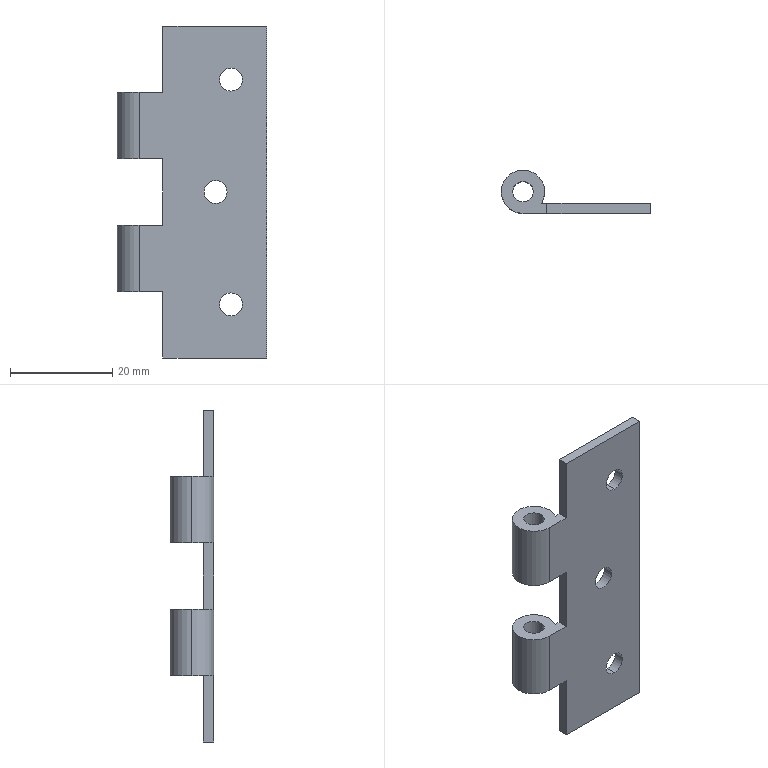Part | NX | features BREP 1 | 1 solid | 28 faces | box 29.25 x 8.5 x 65 mm | volume 3806 mm3 | cylinder 16 | plane 12 | commonest cylinder face diameters 4.5 x6 8.5 x6 4 x4
STEP:
#1=CARTESIAN_POINT('',(17.25,0.,-32.5));
#2=VERTEX_POINT('',#1);
#3=CARTESIAN_POINT('',(12.75,0.,-32.5));
#4=VERTEX_POINT('',#3);
#5=CARTESIAN_POINT('',(15.,0.,-32.5));
#6=DIRECTION('',(0.,1.,0.));
#7=DIRECTION('',(-1.,0.,0.));
#8=AXIS2_PLACEMENT_3D('',#5,#6,#7);
#9=CIRCLE('',#8,2.25);
#10=EDGE_CURVE('',#2,#4,#9,.T.);
#11=ORIENTED_EDGE('',*,*,#10,.F.);
#12=CARTESIAN_POINT('',(17.25,2.,-32.5));
#13=VERTEX_POINT('',#12);
#14=CARTESIAN_POINT('',(17.25,0.,-32.5));
#15=DIRECTION('',(0.,1.,0.));
#16=VECTOR('',#15,1000.);
#17=LINE('',#14,#16);
#18=EDGE_CURVE('',#2,#13,#17,.T.);
#19=ORIENTED_EDGE('',*,*,#18,.T.);
#20=CARTESIAN_POINT('',(12.75,2.,-32.5));
#21=VERTEX_POINT('',#20);
#22=CARTESIAN_POINT('',(15.,2.,-32.5));
#23=DIRECTION('',(0.,1.,0.));
#24=DIRECTION('',(-1.,0.,0.));
#25=AXIS2_PLACEMENT_3D('',#22,#23,#24);
#26=CIRCLE('',#25,2.25);
#27=EDGE_CURVE('',#13,#21,#26,.T.);
#28=ORIENTED_EDGE('',*,*,#27,.T.);
#29=CARTESIAN_POINT('',(12.75,0.,-32.5));
#30=DIRECTION('',(0.,1.,0.));
#31=VECTOR('',#30,1000.);
#32=LINE('',#29,#31);
#33=EDGE_CURVE('',#4,#21,#32,.T.);
#34=ORIENTED_EDGE('',*,*,#33,.F.);
#35=EDGE_LOOP('',(#11,#19,#28,#34));
#36=FACE_BOUND('',#35,.T.);
#37=CARTESIAN_POINT('',(15.,0.,-32.5));
#38=DIRECTION('',(0.,1.,0.));
#39=DIRECTION('',(-1.,0.,0.));
#40=AXIS2_PLACEMENT_3D('',#37,#38,#39);
#41=CYLINDRICAL_SURFACE('',#40,2.25);
#42=ADVANCED_FACE('',(#36),#41,.F.);
#43=CARTESIAN_POINT('',(18.,2.,-12.75));
#44=VERTEX_POINT('',#43);
#45=CARTESIAN_POINT('',(18.,2.,-8.25));
#46=VERTEX_POINT('',#45);
#47=CARTESIAN_POINT('',(18.,2.,-10.5));
#48=DIRECTION('',(0.,1.,0.));
#49=DIRECTION('',(0.,0.,1.));
#50=AXIS2_PLACEMENT_3D('',#47,#48,#49);
#51=CIRCLE('',#50,2.25);
#52=EDGE_CURVE('',#44,#46,#51,.T.);
#53=ORIENTED_EDGE('',*,*,#52,.T.);
#54=CARTESIAN_POINT('',(18.,0.,-8.25));
#55=VERTEX_POINT('',#54);
#56=CARTESIAN_POINT('',(18.,2.,-8.25));
#57=DIRECTION('',(0.,-1.,0.));
#58=VECTOR('',#57,1000.);
#59=LINE('',#56,#58);
#60=EDGE_CURVE('',#46,#55,#59,.T.);
#61=ORIENTED_EDGE('',*,*,#60,.T.);
#62=CARTESIAN_POINT('',(18.,0.,-12.75));
#63=VERTEX_POINT('',#62);
#64=CARTESIAN_POINT('',(18.,0.,-10.5));
#65=DIRECTION('',(0.,1.,0.));
#66=DIRECTION('',(0.,0.,1.));
#67=AXIS2_PLACEMENT_3D('',#64,#65,#66);
#68=CIRCLE('',#67,2.25);
#69=EDGE_CURVE('',#63,#55,#68,.T.);
#70=ORIENTED_EDGE('',*,*,#69,.F.);
#71=CARTESIAN_POINT('',(18.,2.,-12.75));
#72=DIRECTION('',(0.,-1.,0.));
#73=VECTOR('',#72,1000.);
#74=LINE('',#71,#73);
#75=EDGE_CURVE('',#44,#63,#74,.T.);
#76=ORIENTED_EDGE('',*,*,#75,.F.);
#77=EDGE_LOOP('',(#53,#61,#70,#76));
#78=FACE_BOUND('',#77,.T.);
#79=CARTESIAN_POINT('',(18.,2.,-10.5));
#80=DIRECTION('',(0.,-1.,0.));
#81=DIRECTION('',(0.,0.,-1.));
#82=AXIS2_PLACEMENT_3D('',#79,#80,#81);
#83=CYLINDRICAL_SURFACE('',#82,2.25);
#84=ADVANCED_FACE('',(#78),#83,.F.);
#85=CARTESIAN_POINT('',(18.,2.,-56.75));
#86=VERTEX_POINT('',#85);
#87=CARTESIAN_POINT('',(18.,2.,-52.25));
#88=VERTEX_POINT('',#87);
#89=CARTESIAN_POINT('',(18.,2.,-54.5));
#90=DIRECTION('',(0.,1.,0.));
#91=DIRECTION('',(0.,0.,1.));
#92=AXIS2_PLACEMENT_3D('',#89,#90,#91);
#93=CIRCLE('',#92,2.25);
#94=EDGE_CURVE('',#86,#88,#93,.T.);
#95=ORIENTED_EDGE('',*,*,#94,.T.);
#96=CARTESIAN_POINT('',(18.,0.,-52.25));
#97=VERTEX_POINT('',#96);
#98=CARTESIAN_POINT('',(18.,2.,-52.25));
#99=DIRECTION('',(0.,-1.,0.));
#100=VECTOR('',#99,1000.);
#101=LINE('',#98,#100);
#102=EDGE_CURVE('',#88,#97,#101,.T.);
#103=ORIENTED_EDGE('',*,*,#102,.T.);
#104=CARTESIAN_POINT('',(18.,0.,-56.75));
#105=VERTEX_POINT('',#104);
#106=CARTESIAN_POINT('',(18.,0.,-54.5));
#107=DIRECTION('',(0.,1.,0.));
#108=DIRECTION('',(0.,0.,1.));
#109=AXIS2_PLACEMENT_3D('',#106,#107,#108);
#110=CIRCLE('',#109,2.25);
#111=EDGE_CURVE('',#105,#97,#110,.T.);
#112=ORIENTED_EDGE('',*,*,#111,.F.);
#113=CARTESIAN_POINT('',(18.,2.,-56.75));
#114=DIRECTION('',(0.,-1.,0.));
#115=VECTOR('',#114,1000.);
#116=LINE('',#113,#115);
#117=EDGE_CURVE('',#86,#105,#116,.T.);
#118=ORIENTED_EDGE('',*,*,#117,.F.);
#119=EDGE_LOOP('',(#95,#103,#112,#118));
#120=FACE_BOUND('',#119,.T.);
#121=CARTESIAN_POINT('',(18.,2.,-54.5));
#122=DIRECTION('',(0.,-1.,0.));
#123=DIRECTION('',(0.,0.,-1.));
#124=AXIS2_PLACEMENT_3D('',#121,#122,#123);
#125=CYLINDRICAL_SURFACE('',#124,2.25);
#126=ADVANCED_FACE('',(#120),#125,.F.);
#127=CARTESIAN_POINT('',(-2.,4.25,-52.));
#128=VERTEX_POINT('',#127);
#129=CARTESIAN_POINT('',(2.,4.25,-52.));
#130=VERTEX_POINT('',#129);
#131=CARTESIAN_POINT('',(0.,4.25,-52.));
#132=DIRECTION('',(0.,0.,1.));
#133=DIRECTION('',(-1.,0.,0.));
#134=AXIS2_PLACEMENT_3D('',#131,#132,#133);
#135=CIRCLE('',#134,2.);
#136=EDGE_CURVE('',#128,#130,#135,.T.);
#137=ORIENTED_EDGE('',*,*,#136,.F.);
#138=CARTESIAN_POINT('',(-2.,4.25,-39.));
#139=VERTEX_POINT('',#138);
#140=CARTESIAN_POINT('',(-2.,4.25,-65.));
#141=DIRECTION('',(0.,0.,1.));
#142=VECTOR('',#141,1000.);
#143=LINE('',#140,#142);
#144=EDGE_CURVE('',#139,#128,#143,.F.);
#145=ORIENTED_EDGE('',*,*,#144,.F.);
#146=CARTESIAN_POINT('',(2.,4.25,-39.));
#147=VERTEX_POINT('',#146);
#148=CARTESIAN_POINT('',(0.,4.25,-39.));
#149=DIRECTION('',(0.,0.,-1.));
#150=DIRECTION('',(1.,0.,0.));
#151=AXIS2_PLACEMENT_3D('',#148,#149,#150);
#152=CIRCLE('',#151,2.);
#153=EDGE_CURVE('',#147,#139,#152,.T.);
#154=ORIENTED_EDGE('',*,*,#153,.F.);
#155=CARTESIAN_POINT('',(2.,4.25,-65.));
#156=DIRECTION('',(0.,0.,1.));
#157=VECTOR('',#156,1000.);
#158=LINE('',#155,#157);
#159=EDGE_CURVE('',#147,#130,#158,.F.);
#160=ORIENTED_EDGE('',*,*,#159,.T.);
#161=EDGE_LOOP('',(#137,#145,#154,#160));
#162=FACE_BOUND('',#161,.T.);
#163=CARTESIAN_POINT('',(0.,4.25,-65.));
#164=DIRECTION('',(0.,0.,1.));
#165=DIRECTION('',(1.,0.,0.));
#166=AXIS2_PLACEMENT_3D('',#163,#164,#165);
#167=CYLINDRICAL_SURFACE('',#166,2.);
#168=ADVANCED_FACE('',(#162),#167,.F.);
#169=CARTESIAN_POINT('',(-2.,4.25,-26.));
#170=VERTEX_POINT('',#169);
#171=CARTESIAN_POINT('',(2.,4.25,-26.));
#172=VERTEX_POINT('',#171);
#173=CARTESIAN_POINT('',(0.,4.25,-26.));
#174=DIRECTION('',(0.,0.,1.));
#175=DIRECTION('',(-1.,0.,0.));
#176=AXIS2_PLACEMENT_3D('',#173,#174,#175);
#177=CIRCLE('',#176,2.);
#178=EDGE_CURVE('',#170,#172,#177,.T.);
#179=ORIENTED_EDGE('',*,*,#178,.F.);
#180=CARTESIAN_POINT('',(-2.,4.25,-13.));
#181=VERTEX_POINT('',#180);
#182=CARTESIAN_POINT('',(-2.,4.25,-65.));
#183=DIRECTION('',(0.,0.,1.));
#184=VECTOR('',#183,1000.);
#185=LINE('',#182,#184);
#186=EDGE_CURVE('',#181,#170,#185,.F.);
#187=ORIENTED_EDGE('',*,*,#186,.F.);
#188=CARTESIAN_POINT('',(2.,4.25,-13.));
#189=VERTEX_POINT('',#188);
#190=CARTESIAN_POINT('',(0.,4.25,-13.));
#191=DIRECTION('',(0.,0.,-1.));
#192=DIRECTION('',(1.,0.,0.));
#193=AXIS2_PLACEMENT_3D('',#190,#191,#192);
#194=CIRCLE('',#193,2.);
#195=EDGE_CURVE('',#189,#181,#194,.T.);
#196=ORIENTED_EDGE('',*,*,#195,.F.);
#197=CARTESIAN_POINT('',(2.,4.25,-65.));
#198=DIRECTION('',(0.,0.,1.));
#199=VECTOR('',#198,1000.);
#200=LINE('',#197,#199);
#201=EDGE_CURVE('',#189,#172,#200,.F.);
#202=ORIENTED_EDGE('',*,*,#201,.T.);
#203=EDGE_LOOP('',(#179,#187,#196,#202));
#204=FACE_BOUND('',#203,.T.);
#205=CARTESIAN_POINT('',(0.,4.25,-65.));
#206=DIRECTION('',(0.,0.,1.));
#207=DIRECTION('',(1.,0.,0.));
#208=AXIS2_PLACEMENT_3D('',#205,#206,#207);
#209=CYLINDRICAL_SURFACE('',#208,2.);
#210=ADVANCED_FACE('',(#204),#209,.F.);
#211=CARTESIAN_POINT('',(4.25,4.25,-52.));
#212=VERTEX_POINT('',#211);
#213=CARTESIAN_POINT('',(-4.25,4.25,-52.));
#214=VERTEX_POINT('',#213);
#215=CARTESIAN_POINT('',(0.,4.25,-52.));
#216=DIRECTION('',(0.,0.,1.));
#217=DIRECTION('',(-1.,0.,0.));
#218=AXIS2_PLACEMENT_3D('',#215,#216,#217);
#219=CIRCLE('',#218,4.25);
#220=EDGE_CURVE('',#212,#214,#219,.T.);
#221=ORIENTED_EDGE('',*,*,#220,.T.);
#222=CARTESIAN_POINT('',(-4.25,4.25,-39.));
#223=VERTEX_POINT('',#222);
#224=CARTESIAN_POINT('',(-4.25,4.25,-65.));
#225=DIRECTION('',(0.,0.,1.));
#226=VECTOR('',#225,1000.);
#227=LINE('',#224,#226);
#228=EDGE_CURVE('',#214,#223,#227,.T.);
#229=ORIENTED_EDGE('',*,*,#228,.T.);
#230=CARTESIAN_POINT('',(4.25,4.25,-39.));
#231=VERTEX_POINT('',#230);
#232=CARTESIAN_POINT('',(0.,4.25,-39.));
#233=DIRECTION('',(0.,0.,-1.));
#234=DIRECTION('',(1.,0.,0.));
#235=AXIS2_PLACEMENT_3D('',#232,#233,#234);
#236=CIRCLE('',#235,4.25);
#237=EDGE_CURVE('',#223,#231,#236,.T.);
#238=ORIENTED_EDGE('',*,*,#237,.T.);
#239=CARTESIAN_POINT('',(4.25,4.25,-65.));
#240=DIRECTION('',(0.,0.,1.));
#241=VECTOR('',#240,1000.);
#242=LINE('',#239,#241);
#243=EDGE_CURVE('',#212,#231,#242,.T.);
#244=ORIENTED_EDGE('',*,*,#243,.F.);
#245=EDGE_LOOP('',(#221,#229,#238,#244));
#246=FACE_BOUND('',#245,.T.);
#247=CARTESIAN_POINT('',(0.,4.25,-65.));
#248=DIRECTION('',(0.,0.,1.));
#249=DIRECTION('',(1.,0.,0.));
#250=AXIS2_PLACEMENT_3D('',#247,#248,#249);
#251=CYLINDRICAL_SURFACE('',#250,4.25);
#252=ADVANCED_FACE('',(#246),#251,.T.);
#253=CARTESIAN_POINT('',(3.606,2.,-52.));
#254=VERTEX_POINT('',#253);
#255=CARTESIAN_POINT('',(0.,4.25,-52.));
#256=DIRECTION('',(0.,0.,1.));
#257=DIRECTION('',(-1.,0.,0.));
#258=AXIS2_PLACEMENT_3D('',#255,#256,#257);
#259=CIRCLE('',#258,4.25);
#260=EDGE_CURVE('',#254,#212,#259,.T.);
#261=ORIENTED_EDGE('',*,*,#260,.T.);
#262=ORIENTED_EDGE('',*,*,#243,.T.);
#263=CARTESIAN_POINT('',(3.606,2.,-39.));
#264=VERTEX_POINT('',#263);
#265=CARTESIAN_POINT('',(0.,4.25,-39.));
#266=DIRECTION('',(0.,0.,-1.));
#267=DIRECTION('',(1.,0.,0.));
#268=AXIS2_PLACEMENT_3D('',#265,#266,#267);
#269=CIRCLE('',#268,4.25);
#270=EDGE_CURVE('',#231,#264,#269,.T.);
#271=ORIENTED_EDGE('',*,*,#270,.T.);
#272=CARTESIAN_POINT('',(3.606,2.,-65.));
#273=DIRECTION('',(0.,0.,1.));
#274=VECTOR('',#273,1000.);
#275=LINE('',#272,#274);
#276=EDGE_CURVE('',#254,#264,#275,.T.);
#277=ORIENTED_EDGE('',*,*,#276,.F.);
#278=EDGE_LOOP('',(#261,#262,#271,#277));
#279=FACE_BOUND('',#278,.T.);
#280=CARTESIAN_POINT('',(0.,4.25,-65.));
#281=DIRECTION('',(0.,0.,1.));
#282=DIRECTION('',(1.,0.,0.));
#283=AXIS2_PLACEMENT_3D('',#280,#281,#282);
#284=CYLINDRICAL_SURFACE('',#283,4.25);
#285=ADVANCED_FACE('',(#279),#284,.T.);
#286=CARTESIAN_POINT('',(4.25,4.25,-26.));
#287=VERTEX_POINT('',#286);
#288=CARTESIAN_POINT('',(-4.25,4.25,-26.));
#289=VERTEX_POINT('',#288);
#290=CARTESIAN_POINT('',(0.,4.25,-26.));
#291=DIRECTION('',(0.,0.,1.));
#292=DIRECTION('',(-1.,0.,0.));
#293=AXIS2_PLACEMENT_3D('',#290,#291,#292);
#294=CIRCLE('',#293,4.25);
#295=EDGE_CURVE('',#287,#289,#294,.T.);
#296=ORIENTED_EDGE('',*,*,#295,.T.);
#297=CARTESIAN_POINT('',(-4.25,4.25,-13.));
#298=VERTEX_POINT('',#297);
#299=CARTESIAN_POINT('',(-4.25,4.25,-65.));
#300=DIRECTION('',(0.,0.,1.));
#301=VECTOR('',#300,1000.);
#302=LINE('',#299,#301);
#303=EDGE_CURVE('',#289,#298,#302,.T.);
#304=ORIENTED_EDGE('',*,*,#303,.T.);
#305=CARTESIAN_POINT('',(4.25,4.25,-13.));
#306=VERTEX_POINT('',#305);
#307=CARTESIAN_POINT('',(0.,4.25,-13.));
#308=DIRECTION('',(0.,0.,-1.));
#309=DIRECTION('',(1.,0.,0.));
#310=AXIS2_PLACEMENT_3D('',#307,#308,#309);
#311=CIRCLE('',#310,4.25);
#312=EDGE_CURVE('',#298,#306,#311,.T.);
#313=ORIENTED_EDGE('',*,*,#312,.T.);
#314=CARTESIAN_POINT('',(4.25,4.25,-65.));
#315=DIRECTION('',(0.,0.,1.));
#316=VECTOR('',#315,1000.);
#317=LINE('',#314,#316);
#318=EDGE_CURVE('',#287,#306,#317,.T.);
#319=ORIENTED_EDGE('',*,*,#318,.F.);
#320=EDGE_LOOP('',(#296,#304,#313,#319));
#321=FACE_BOUND('',#320,.T.);
#322=CARTESIAN_POINT('',(0.,4.25,-65.));
#323=DIRECTION('',(0.,0.,1.));
#324=DIRECTION('',(1.,0.,0.));
#325=AXIS2_PLACEMENT_3D('',#322,#323,#324);
#326=CYLINDRICAL_SURFACE('',#325,4.25);
#327=ADVANCED_FACE('',(#321),#326,.T.);
#328=CARTESIAN_POINT('',(3.606,2.,-26.));
#329=VERTEX_POINT('',#328);
#330=CARTESIAN_POINT('',(0.,4.25,-26.));
#331=DIRECTION('',(0.,0.,1.));
#332=DIRECTION('',(-1.,0.,0.));
#333=AXIS2_PLACEMENT_3D('',#330,#331,#332);
#334=CIRCLE('',#333,4.25);
#335=EDGE_CURVE('',#329,#287,#334,.T.);
#336=ORIENTED_EDGE('',*,*,#335,.T.);
#337=ORIENTED_EDGE('',*,*,#318,.T.);
#338=CARTESIAN_POINT('',(3.606,2.,-13.));
#339=VERTEX_POINT('',#338);
#340=CARTESIAN_POINT('',(0.,4.25,-13.));
#341=DIRECTION('',(0.,0.,-1.));
#342=DIRECTION('',(1.,0.,0.));
#343=AXIS2_PLACEMENT_3D('',#340,#341,#342);
#344=CIRCLE('',#343,4.25);
#345=EDGE_CURVE('',#306,#339,#344,.T.);
#346=ORIENTED_EDGE('',*,*,#345,.T.);
#347=CARTESIAN_POINT('',(3.606,2.,-65.));
#348=DIRECTION('',(0.,0.,1.));
#349=VECTOR('',#348,1000.);
#350=LINE('',#347,#349);
#351=EDGE_CURVE('',#329,#339,#350,.T.);
#352=ORIENTED_EDGE('',*,*,#351,.F.);
#353=EDGE_LOOP('',(#336,#337,#346,#352));
#354=FACE_BOUND('',#353,.T.);
#355=CARTESIAN_POINT('',(0.,4.25,-65.));
#356=DIRECTION('',(0.,0.,1.));
#357=DIRECTION('',(1.,0.,0.));
#358=AXIS2_PLACEMENT_3D('',#355,#356,#357);
#359=CYLINDRICAL_SURFACE('',#358,4.25);
#360=ADVANCED_FACE('',(#354),#359,.T.);
#361=CARTESIAN_POINT('',(4.675,2.,-13.));
#362=VERTEX_POINT('',#361);
#363=CARTESIAN_POINT('',(25.,2.,-13.));
#364=DIRECTION('',(1.,0.,0.));
#365=VECTOR('',#364,1000.);
#366=LINE('',#363,#365);
#367=EDGE_CURVE('',#339,#362,#366,.T.);
#368=ORIENTED_EDGE('',*,*,#367,.T.);
#369=CARTESIAN_POINT('',(4.675,2.,0.));
#370=VERTEX_POINT('',#369);
#371=CARTESIAN_POINT('',(4.675,2.,-65.));
#372=DIRECTION('',(0.,0.,1.));
#373=VECTOR('',#372,1000.);
#374=LINE('',#371,#373);
#375=EDGE_CURVE('',#362,#370,#374,.T.);
#376=ORIENTED_EDGE('',*,*,#375,.T.);
#377=CARTESIAN_POINT('',(25.,2.,0.));
#378=VERTEX_POINT('',#377);
#379=CARTESIAN_POINT('',(25.,2.,0.));
#380=DIRECTION('',(-1.,0.,0.));
#381=VECTOR('',#380,1000.);
#382=LINE('',#379,#381);
#383=EDGE_CURVE('',#378,#370,#382,.T.);
#384=ORIENTED_EDGE('',*,*,#383,.F.);
#385=CARTESIAN_POINT('',(25.,2.,-65.));
#386=VERTEX_POINT('',#385);
#387=CARTESIAN_POINT('',(25.,2.,-65.));
#388=DIRECTION('',(0.,0.,1.));
#389=VECTOR('',#388,1000.);
#390=LINE('',#387,#389);
#391=EDGE_CURVE('',#386,#378,#390,.T.);
#392=ORIENTED_EDGE('',*,*,#391,.F.);
#393=CARTESIAN_POINT('',(4.675,2.,-65.));
#394=VERTEX_POINT('',#393);
#395=CARTESIAN_POINT('',(25.,2.,-65.));
#396=DIRECTION('',(-1.,0.,0.));
#397=VECTOR('',#396,1000.);
#398=LINE('',#395,#397);
#399=EDGE_CURVE('',#386,#394,#398,.T.);
#400=ORIENTED_EDGE('',*,*,#399,.T.);
#401=CARTESIAN_POINT('',(4.675,2.,-52.));
#402=VERTEX_POINT('',#401);
#403=CARTESIAN_POINT('',(4.675,2.,-65.));
#404=DIRECTION('',(0.,0.,1.));
#405=VECTOR('',#404,1000.);
#406=LINE('',#403,#405);
#407=EDGE_CURVE('',#394,#402,#406,.T.);
#408=ORIENTED_EDGE('',*,*,#407,.T.);
#409=CARTESIAN_POINT('',(25.,2.,-52.));
#410=DIRECTION('',(-1.,0.,0.));
#411=VECTOR('',#410,1000.);
#412=LINE('',#409,#411);
#413=EDGE_CURVE('',#402,#254,#412,.T.);
#414=ORIENTED_EDGE('',*,*,#413,.T.);
#415=ORIENTED_EDGE('',*,*,#276,.T.);
#416=CARTESIAN_POINT('',(4.675,2.,-39.));
#417=VERTEX_POINT('',#416);
#418=CARTESIAN_POINT('',(25.,2.,-39.));
#419=DIRECTION('',(1.,0.,0.));
#420=VECTOR('',#419,1000.);
#421=LINE('',#418,#420);
#422=EDGE_CURVE('',#264,#417,#421,.T.);
#423=ORIENTED_EDGE('',*,*,#422,.T.);
#424=CARTESIAN_POINT('',(4.675,2.,-26.));
#425=VERTEX_POINT('',#424);
#426=CARTESIAN_POINT('',(4.675,2.,-65.));
#427=DIRECTION('',(0.,0.,1.));
#428=VECTOR('',#427,1000.);
#429=LINE('',#426,#428);
#430=EDGE_CURVE('',#417,#425,#429,.T.);
#431=ORIENTED_EDGE('',*,*,#430,.T.);
#432=CARTESIAN_POINT('',(25.,2.,-26.));
#433=DIRECTION('',(-1.,0.,0.));
#434=VECTOR('',#433,1000.);
#435=LINE('',#432,#434);
#436=EDGE_CURVE('',#425,#329,#435,.T.);
#437=ORIENTED_EDGE('',*,*,#436,.T.);
#438=ORIENTED_EDGE('',*,*,#351,.T.);
#439=EDGE_LOOP('',(#368,#376,#384,#392,#400,#408,#414,#415,#423,#431,#437,#438));
#440=FACE_BOUND('',#439,.T.);
#441=CARTESIAN_POINT('',(15.,2.,-32.5));
#442=DIRECTION('',(0.,1.,0.));
#443=DIRECTION('',(-1.,0.,0.));
#444=AXIS2_PLACEMENT_3D('',#441,#442,#443);
#445=CIRCLE('',#444,2.25);
#446=EDGE_CURVE('',#21,#13,#445,.T.);
#447=ORIENTED_EDGE('',*,*,#446,.F.);
#448=ORIENTED_EDGE('',*,*,#27,.F.);
#449=EDGE_LOOP('',(#447,#448));
#450=FACE_BOUND('',#449,.T.);
#451=ORIENTED_EDGE('',*,*,#94,.F.);
#452=CARTESIAN_POINT('',(18.,2.,-54.5));
#453=DIRECTION('',(0.,1.,0.));
#454=DIRECTION('',(0.,0.,1.));
#455=AXIS2_PLACEMENT_3D('',#452,#453,#454);
#456=CIRCLE('',#455,2.25);
#457=EDGE_CURVE('',#88,#86,#456,.T.);
#458=ORIENTED_EDGE('',*,*,#457,.F.);
#459=EDGE_LOOP('',(#451,#458));
#460=FACE_BOUND('',#459,.T.);
#461=ORIENTED_EDGE('',*,*,#52,.F.);
#462=CARTESIAN_POINT('',(18.,2.,-10.5));
#463=DIRECTION('',(0.,1.,0.));
#464=DIRECTION('',(0.,0.,1.));
#465=AXIS2_PLACEMENT_3D('',#462,#463,#464);
#466=CIRCLE('',#465,2.25);
#467=EDGE_CURVE('',#46,#44,#466,.T.);
#468=ORIENTED_EDGE('',*,*,#467,.F.);
#469=EDGE_LOOP('',(#461,#468));
#470=FACE_BOUND('',#469,.T.);
#471=CARTESIAN_POINT('',(25.,2.,-65.));
#472=DIRECTION('',(0.,1.,0.));
#473=DIRECTION('',(1.,0.,0.));
#474=AXIS2_PLACEMENT_3D('',#471,#472,#473);
#475=PLANE('',#474);
#476=ADVANCED_FACE('',(#440,#450,#460,#470),#475,.T.);
#477=CARTESIAN_POINT('',(4.675,0.,0.));
#478=VERTEX_POINT('',#477);
#479=CARTESIAN_POINT('',(25.,0.,0.));
#480=VERTEX_POINT('',#479);
#481=CARTESIAN_POINT('',(0.,0.,0.));
#482=DIRECTION('',(1.,0.,0.));
#483=VECTOR('',#482,1000.);
#484=LINE('',#481,#483);
#485=EDGE_CURVE('',#478,#480,#484,.T.);
#486=ORIENTED_EDGE('',*,*,#485,.F.);
#487=CARTESIAN_POINT('',(4.675,0.,-13.));
#488=VERTEX_POINT('',#487);
#489=CARTESIAN_POINT('',(4.675,0.,0.));
#490=DIRECTION('',(0.,0.,-1.));
#491=VECTOR('',#490,1000.);
#492=LINE('',#489,#491);
#493=EDGE_CURVE('',#478,#488,#492,.T.);
#494=ORIENTED_EDGE('',*,*,#493,.T.);
#495=CARTESIAN_POINT('',(0.,0.,-13.));
#496=VERTEX_POINT('',#495);
#497=CARTESIAN_POINT('',(4.675,0.,-13.));
#498=DIRECTION('',(-1.,0.,0.));
#499=VECTOR('',#498,1000.);
#500=LINE('',#497,#499);
#501=EDGE_CURVE('',#488,#496,#500,.T.);
#502=ORIENTED_EDGE('',*,*,#501,.T.);
#503=CARTESIAN_POINT('',(0.,0.,-26.));
#504=VERTEX_POINT('',#503);
#505=CARTESIAN_POINT('',(0.,0.,-65.));
#506=DIRECTION('',(0.,0.,1.));
#507=VECTOR('',#506,1000.);
#508=LINE('',#505,#507);
#509=EDGE_CURVE('',#504,#496,#508,.T.);
#510=ORIENTED_EDGE('',*,*,#509,.F.);
#511=CARTESIAN_POINT('',(4.675,0.,-26.));
#512=VERTEX_POINT('',#511);
#513=CARTESIAN_POINT('',(-8.888,0.,-26.));
#514=DIRECTION('',(1.,0.,0.));
#515=VECTOR('',#514,1000.);
#516=LINE('',#513,#515);
#517=EDGE_CURVE('',#504,#512,#516,.T.);
#518=ORIENTED_EDGE('',*,*,#517,.T.);
#519=CARTESIAN_POINT('',(4.675,0.,-39.));
#520=VERTEX_POINT('',#519);
#521=CARTESIAN_POINT('',(4.675,0.,-26.));
#522=DIRECTION('',(0.,0.,-1.));
#523=VECTOR('',#522,1000.);
#524=LINE('',#521,#523);
#525=EDGE_CURVE('',#512,#520,#524,.T.);
#526=ORIENTED_EDGE('',*,*,#525,.T.);
#527=CARTESIAN_POINT('',(0.,0.,-39.));
#528=VERTEX_POINT('',#527);
#529=CARTESIAN_POINT('',(4.675,0.,-39.));
#530=DIRECTION('',(-1.,0.,0.));
#531=VECTOR('',#530,1000.);
#532=LINE('',#529,#531);
#533=EDGE_CURVE('',#520,#528,#532,.T.);
#534=ORIENTED_EDGE('',*,*,#533,.T.);
#535=CARTESIAN_POINT('',(0.,0.,-52.));
#536=VERTEX_POINT('',#535);
#537=CARTESIAN_POINT('',(0.,0.,-65.));
#538=DIRECTION('',(0.,0.,1.));
#539=VECTOR('',#538,1000.);
#540=LINE('',#537,#539);
#541=EDGE_CURVE('',#536,#528,#540,.T.);
#542=ORIENTED_EDGE('',*,*,#541,.F.);
#543=CARTESIAN_POINT('',(4.675,0.,-52.));
#544=VERTEX_POINT('',#543);
#545=CARTESIAN_POINT('',(-8.888,0.,-52.));
#546=DIRECTION('',(1.,0.,0.));
#547=VECTOR('',#546,1000.);
#548=LINE('',#545,#547);
#549=EDGE_CURVE('',#536,#544,#548,.T.);
#550=ORIENTED_EDGE('',*,*,#549,.T.);
#551=CARTESIAN_POINT('',(4.675,0.,-65.));
#552=VERTEX_POINT('',#551);
#553=CARTESIAN_POINT('',(4.675,0.,-52.));
#554=DIRECTION('',(0.,0.,-1.));
#555=VECTOR('',#554,1000.);
#556=LINE('',#553,#555);
#557=EDGE_CURVE('',#544,#552,#556,.T.);
#558=ORIENTED_EDGE('',*,*,#557,.T.);
#559=CARTESIAN_POINT('',(25.,0.,-65.));
#560=VERTEX_POINT('',#559);
#561=CARTESIAN_POINT('',(0.,0.,-65.));
#562=DIRECTION('',(1.,0.,0.));
#563=VECTOR('',#562,1000.);
#564=LINE('',#561,#563);
#565=EDGE_CURVE('',#552,#560,#564,.T.);
#566=ORIENTED_EDGE('',*,*,#565,.T.);
#567=CARTESIAN_POINT('',(25.,0.,-65.));
#568=DIRECTION('',(0.,0.,1.));
#569=VECTOR('',#568,1000.);
#570=LINE('',#567,#569);
#571=EDGE_CURVE('',#560,#480,#570,.T.);
#572=ORIENTED_EDGE('',*,*,#571,.T.);
#573=EDGE_LOOP('',(#486,#494,#502,#510,#518,#526,#534,#542,#550,#558,#566,#572));
#574=FACE_BOUND('',#573,.T.);
#575=CARTESIAN_POINT('',(15.,0.,-32.5));
#576=DIRECTION('',(0.,1.,0.));
#577=DIRECTION('',(-1.,0.,0.));
#578=AXIS2_PLACEMENT_3D('',#575,#576,#577);
#579=CIRCLE('',#578,2.25);
#580=EDGE_CURVE('',#4,#2,#579,.T.);
#581=ORIENTED_EDGE('',*,*,#580,.T.);
#582=ORIENTED_EDGE('',*,*,#10,.T.);
#583=EDGE_LOOP('',(#581,#582));
#584=FACE_BOUND('',#583,.T.);
#585=ORIENTED_EDGE('',*,*,#111,.T.);
#586=CARTESIAN_POINT('',(18.,0.,-54.5));
#587=DIRECTION('',(0.,1.,0.));
#588=DIRECTION('',(0.,0.,1.));
#589=AXIS2_PLACEMENT_3D('',#586,#587,#588);
#590=CIRCLE('',#589,2.25);
#591=EDGE_CURVE('',#97,#105,#590,.T.);
#592=ORIENTED_EDGE('',*,*,#591,.T.);
#593=EDGE_LOOP('',(#585,#592));
#594=FACE_BOUND('',#593,.T.);
#595=ORIENTED_EDGE('',*,*,#69,.T.);
#596=CARTESIAN_POINT('',(18.,0.,-10.5));
#597=DIRECTION('',(0.,1.,0.));
#598=DIRECTION('',(0.,0.,1.));
#599=AXIS2_PLACEMENT_3D('',#596,#597,#598);
#600=CIRCLE('',#599,2.25);
#601=EDGE_CURVE('',#55,#63,#600,.T.);
#602=ORIENTED_EDGE('',*,*,#601,.T.);
#603=EDGE_LOOP('',(#595,#602));
#604=FACE_BOUND('',#603,.T.);
#605=CARTESIAN_POINT('',(0.,0.,-65.));
#606=DIRECTION('',(0.,-1.,0.));
#607=DIRECTION('',(0.,0.,-1.));
#608=AXIS2_PLACEMENT_3D('',#605,#606,#607);
#609=PLANE('',#608);
#610=ADVANCED_FACE('',(#574,#584,#594,#604),#609,.T.);
#611=ORIENTED_EDGE('',*,*,#303,.F.);
#612=CARTESIAN_POINT('',(0.,4.25,-26.));
#613=DIRECTION('',(0.,0.,1.));
#614=DIRECTION('',(-1.,0.,0.));
#615=AXIS2_PLACEMENT_3D('',#612,#613,#614);
#616=CIRCLE('',#615,4.25);
#617=EDGE_CURVE('',#289,#504,#616,.T.);
#618=ORIENTED_EDGE('',*,*,#617,.T.);
#619=ORIENTED_EDGE('',*,*,#509,.T.);
#620=CARTESIAN_POINT('',(0.,4.25,-13.));
#621=DIRECTION('',(0.,0.,-1.));
#622=DIRECTION('',(1.,0.,0.));
#623=AXIS2_PLACEMENT_3D('',#620,#621,#622);
#624=CIRCLE('',#623,4.25);
#625=EDGE_CURVE('',#496,#298,#624,.T.);
#626=ORIENTED_EDGE('',*,*,#625,.T.);
#627=EDGE_LOOP('',(#611,#618,#619,#626));
#628=FACE_BOUND('',#627,.T.);
#629=CARTESIAN_POINT('',(0.,4.25,-65.));
#630=DIRECTION('',(0.,0.,1.));
#631=DIRECTION('',(1.,0.,0.));
#632=AXIS2_PLACEMENT_3D('',#629,#630,#631);
#633=CYLINDRICAL_SURFACE('',#632,4.25);
#634=ADVANCED_FACE('',(#628),#633,.T.);
#635=ORIENTED_EDGE('',*,*,#228,.F.);
#636=CARTESIAN_POINT('',(0.,4.25,-52.));
#637=DIRECTION('',(0.,0.,1.));
#638=DIRECTION('',(-1.,0.,0.));
#639=AXIS2_PLACEMENT_3D('',#636,#637,#638);
#640=CIRCLE('',#639,4.25);
#641=EDGE_CURVE('',#214,#536,#640,.T.);
#642=ORIENTED_EDGE('',*,*,#641,.T.);
#643=ORIENTED_EDGE('',*,*,#541,.T.);
#644=CARTESIAN_POINT('',(0.,4.25,-39.));
#645=DIRECTION('',(0.,0.,-1.));
#646=DIRECTION('',(1.,0.,0.));
#647=AXIS2_PLACEMENT_3D('',#644,#645,#646);
#648=CIRCLE('',#647,4.25);
#649=EDGE_CURVE('',#528,#223,#648,.T.);
#650=ORIENTED_EDGE('',*,*,#649,.T.);
#651=EDGE_LOOP('',(#635,#642,#643,#650));
#652=FACE_BOUND('',#651,.T.);
#653=CARTESIAN_POINT('',(0.,4.25,-65.));
#654=DIRECTION('',(0.,0.,1.));
#655=DIRECTION('',(1.,0.,0.));
#656=AXIS2_PLACEMENT_3D('',#653,#654,#655);
#657=CYLINDRICAL_SURFACE('',#656,4.25);
#658=ADVANCED_FACE('',(#652),#657,.T.);
#659=CARTESIAN_POINT('',(4.675,8.5,-65.));
#660=DIRECTION('',(0.,-1.,0.));
#661=VECTOR('',#660,1000.);
#662=LINE('',#659,#661);
#663=EDGE_CURVE('',#394,#552,#662,.T.);
#664=ORIENTED_EDGE('',*,*,#663,.F.);
#665=ORIENTED_EDGE('',*,*,#399,.F.);
#666=CARTESIAN_POINT('',(25.,0.,-65.));
#667=DIRECTION('',(0.,1.,0.));
#668=VECTOR('',#667,1000.);
#669=LINE('',#666,#668);
#670=EDGE_CURVE('',#560,#386,#669,.T.);
#671=ORIENTED_EDGE('',*,*,#670,.F.);
#672=ORIENTED_EDGE('',*,*,#565,.F.);
#673=EDGE_LOOP('',(#664,#665,#671,#672));
#674=FACE_BOUND('',#673,.T.);
#675=CARTESIAN_POINT('',(0.,4.25,-65.));
#676=DIRECTION('',(0.,0.,1.));
#677=DIRECTION('',(1.,0.,0.));
#678=AXIS2_PLACEMENT_3D('',#675,#676,#677);
#679=PLANE('',#678);
#680=ADVANCED_FACE('',(#674),#679,.F.);
#681=ORIENTED_EDGE('',*,*,#383,.T.);
#682=CARTESIAN_POINT('',(4.675,8.5,0.));
#683=DIRECTION('',(0.,-1.,0.));
#684=VECTOR('',#683,1000.);
#685=LINE('',#682,#684);
#686=EDGE_CURVE('',#370,#478,#685,.T.);
#687=ORIENTED_EDGE('',*,*,#686,.T.);
#688=ORIENTED_EDGE('',*,*,#485,.T.);
#689=CARTESIAN_POINT('',(25.,0.,0.));
#690=DIRECTION('',(0.,1.,0.));
#691=VECTOR('',#690,1000.);
#692=LINE('',#689,#691);
#693=EDGE_CURVE('',#480,#378,#692,.T.);
#694=ORIENTED_EDGE('',*,*,#693,.T.);
#695=EDGE_LOOP('',(#681,#687,#688,#694));
#696=FACE_BOUND('',#695,.T.);
#697=CARTESIAN_POINT('',(0.,4.25,0.));
#698=DIRECTION('',(0.,0.,1.));
#699=DIRECTION('',(1.,0.,0.));
#700=AXIS2_PLACEMENT_3D('',#697,#698,#699);
#701=PLANE('',#700);
#702=ADVANCED_FACE('',(#696),#701,.T.);
#703=ORIENTED_EDGE('',*,*,#693,.F.);
#704=ORIENTED_EDGE('',*,*,#571,.F.);
#705=ORIENTED_EDGE('',*,*,#670,.T.);
#706=ORIENTED_EDGE('',*,*,#391,.T.);
#707=EDGE_LOOP('',(#703,#704,#705,#706));
#708=FACE_BOUND('',#707,.T.);
#709=CARTESIAN_POINT('',(25.,0.,-65.));
#710=DIRECTION('',(1.,0.,0.));
#711=DIRECTION('',(0.,1.,0.));
#712=AXIS2_PLACEMENT_3D('',#709,#710,#711);
#713=PLANE('',#712);
#714=ADVANCED_FACE('',(#708),#713,.T.);
#715=ORIENTED_EDGE('',*,*,#260,.F.);
#716=ORIENTED_EDGE('',*,*,#413,.F.);
#717=CARTESIAN_POINT('',(4.675,8.5,-52.));
#718=DIRECTION('',(0.,-1.,0.));
#719=VECTOR('',#718,1000.);
#720=LINE('',#717,#719);
#721=EDGE_CURVE('',#402,#544,#720,.T.);
#722=ORIENTED_EDGE('',*,*,#721,.T.);
#723=ORIENTED_EDGE('',*,*,#549,.F.);
#724=ORIENTED_EDGE('',*,*,#641,.F.);
#725=ORIENTED_EDGE('',*,*,#220,.F.);
#726=EDGE_LOOP('',(#715,#716,#722,#723,#724,#725));
#727=FACE_BOUND('',#726,.T.);
#728=CARTESIAN_POINT('',(0.,4.25,-52.));
#729=DIRECTION('',(0.,0.,1.));
#730=DIRECTION('',(-1.,0.,0.));
#731=AXIS2_PLACEMENT_3D('',#728,#729,#730);
#732=CIRCLE('',#731,2.);
#733=EDGE_CURVE('',#130,#128,#732,.T.);
#734=ORIENTED_EDGE('',*,*,#733,.T.);
#735=ORIENTED_EDGE('',*,*,#136,.T.);
#736=EDGE_LOOP('',(#734,#735));
#737=FACE_BOUND('',#736,.T.);
#738=CARTESIAN_POINT('',(-8.888,8.5,-52.));
#739=DIRECTION('',(0.,0.,-1.));
#740=DIRECTION('',(0.,-1.,0.));
#741=AXIS2_PLACEMENT_3D('',#738,#739,#740);
#742=PLANE('',#741);
#743=ADVANCED_FACE('',(#727,#737),#742,.T.);
#744=ORIENTED_EDGE('',*,*,#663,.T.);
#745=ORIENTED_EDGE('',*,*,#557,.F.);
#746=ORIENTED_EDGE('',*,*,#721,.F.);
#747=ORIENTED_EDGE('',*,*,#407,.F.);
#748=EDGE_LOOP('',(#744,#745,#746,#747));
#749=FACE_BOUND('',#748,.T.);
#750=CARTESIAN_POINT('',(4.675,8.5,-52.));
#751=DIRECTION('',(-1.,0.,0.));
#752=DIRECTION('',(0.,0.,1.));
#753=AXIS2_PLACEMENT_3D('',#750,#751,#752);
#754=PLANE('',#753);
#755=ADVANCED_FACE('',(#749),#754,.T.);
#756=ORIENTED_EDGE('',*,*,#335,.F.);
#757=ORIENTED_EDGE('',*,*,#436,.F.);
#758=CARTESIAN_POINT('',(4.675,8.5,-26.));
#759=DIRECTION('',(0.,-1.,0.));
#760=VECTOR('',#759,1000.);
#761=LINE('',#758,#760);
#762=EDGE_CURVE('',#425,#512,#761,.T.);
#763=ORIENTED_EDGE('',*,*,#762,.T.);
#764=ORIENTED_EDGE('',*,*,#517,.F.);
#765=ORIENTED_EDGE('',*,*,#617,.F.);
#766=ORIENTED_EDGE('',*,*,#295,.F.);
#767=EDGE_LOOP('',(#756,#757,#763,#764,#765,#766));
#768=FACE_BOUND('',#767,.T.);
#769=CARTESIAN_POINT('',(0.,4.25,-26.));
#770=DIRECTION('',(0.,0.,1.));
#771=DIRECTION('',(-1.,0.,0.));
#772=AXIS2_PLACEMENT_3D('',#769,#770,#771);
#773=CIRCLE('',#772,2.);
#774=EDGE_CURVE('',#172,#170,#773,.T.);
#775=ORIENTED_EDGE('',*,*,#774,.T.);
#776=ORIENTED_EDGE('',*,*,#178,.T.);
#777=EDGE_LOOP('',(#775,#776));
#778=FACE_BOUND('',#777,.T.);
#779=CARTESIAN_POINT('',(-8.888,8.5,-26.));
#780=DIRECTION('',(0.,0.,-1.));
#781=DIRECTION('',(0.,-1.,0.));
#782=AXIS2_PLACEMENT_3D('',#779,#780,#781);
#783=PLANE('',#782);
#784=ADVANCED_FACE('',(#768,#778),#783,.T.);
#785=ORIENTED_EDGE('',*,*,#533,.F.);
#786=CARTESIAN_POINT('',(4.675,8.5,-39.));
#787=DIRECTION('',(0.,-1.,0.));
#788=VECTOR('',#787,1000.);
#789=LINE('',#786,#788);
#790=EDGE_CURVE('',#417,#520,#789,.T.);
#791=ORIENTED_EDGE('',*,*,#790,.F.);
#792=ORIENTED_EDGE('',*,*,#422,.F.);
#793=ORIENTED_EDGE('',*,*,#270,.F.);
#794=ORIENTED_EDGE('',*,*,#237,.F.);
#795=ORIENTED_EDGE('',*,*,#649,.F.);
#796=EDGE_LOOP('',(#785,#791,#792,#793,#794,#795));
#797=FACE_BOUND('',#796,.T.);
#798=ORIENTED_EDGE('',*,*,#153,.T.);
#799=CARTESIAN_POINT('',(0.,4.25,-39.));
#800=DIRECTION('',(0.,0.,-1.));
#801=DIRECTION('',(1.,0.,0.));
#802=AXIS2_PLACEMENT_3D('',#799,#800,#801);
#803=CIRCLE('',#802,2.);
#804=EDGE_CURVE('',#139,#147,#803,.T.);
#805=ORIENTED_EDGE('',*,*,#804,.T.);
#806=EDGE_LOOP('',(#798,#805));
#807=FACE_BOUND('',#806,.T.);
#808=CARTESIAN_POINT('',(4.675,8.5,-39.));
#809=DIRECTION('',(0.,0.,1.));
#810=DIRECTION('',(1.,0.,0.));
#811=AXIS2_PLACEMENT_3D('',#808,#809,#810);
#812=PLANE('',#811);
#813=ADVANCED_FACE('',(#797,#807),#812,.T.);
#814=ORIENTED_EDGE('',*,*,#790,.T.);
#815=ORIENTED_EDGE('',*,*,#525,.F.);
#816=ORIENTED_EDGE('',*,*,#762,.F.);
#817=ORIENTED_EDGE('',*,*,#430,.F.);
#818=EDGE_LOOP('',(#814,#815,#816,#817));
#819=FACE_BOUND('',#818,.T.);
#820=CARTESIAN_POINT('',(4.675,8.5,-26.));
#821=DIRECTION('',(-1.,0.,0.));
#822=DIRECTION('',(0.,1.,0.));
#823=AXIS2_PLACEMENT_3D('',#820,#821,#822);
#824=PLANE('',#823);
#825=ADVANCED_FACE('',(#819),#824,.T.);
#826=ORIENTED_EDGE('',*,*,#186,.T.);
#827=ORIENTED_EDGE('',*,*,#774,.F.);
#828=ORIENTED_EDGE('',*,*,#201,.F.);
#829=CARTESIAN_POINT('',(0.,4.25,-13.));
#830=DIRECTION('',(0.,0.,-1.));
#831=DIRECTION('',(1.,0.,0.));
#832=AXIS2_PLACEMENT_3D('',#829,#830,#831);
#833=CIRCLE('',#832,2.);
#834=EDGE_CURVE('',#181,#189,#833,.T.);
#835=ORIENTED_EDGE('',*,*,#834,.F.);
#836=EDGE_LOOP('',(#826,#827,#828,#835));
#837=FACE_BOUND('',#836,.T.);
#838=CARTESIAN_POINT('',(0.,4.25,-65.));
#839=DIRECTION('',(0.,0.,1.));
#840=DIRECTION('',(1.,0.,0.));
#841=AXIS2_PLACEMENT_3D('',#838,#839,#840);
#842=CYLINDRICAL_SURFACE('',#841,2.);
#843=ADVANCED_FACE('',(#837),#842,.F.);
#844=ORIENTED_EDGE('',*,*,#501,.F.);
#845=CARTESIAN_POINT('',(4.675,8.5,-13.));
#846=DIRECTION('',(0.,-1.,0.));
#847=VECTOR('',#846,1000.);
#848=LINE('',#845,#847);
#849=EDGE_CURVE('',#362,#488,#848,.T.);
#850=ORIENTED_EDGE('',*,*,#849,.F.);
#851=ORIENTED_EDGE('',*,*,#367,.F.);
#852=ORIENTED_EDGE('',*,*,#345,.F.);
#853=ORIENTED_EDGE('',*,*,#312,.F.);
#854=ORIENTED_EDGE('',*,*,#625,.F.);
#855=EDGE_LOOP('',(#844,#850,#851,#852,#853,#854));
#856=FACE_BOUND('',#855,.T.);
#857=ORIENTED_EDGE('',*,*,#195,.T.);
#858=ORIENTED_EDGE('',*,*,#834,.T.);
#859=EDGE_LOOP('',(#857,#858));
#860=FACE_BOUND('',#859,.T.);
#861=CARTESIAN_POINT('',(4.675,8.5,-13.));
#862=DIRECTION('',(0.,0.,1.));
#863=DIRECTION('',(1.,0.,0.));
#864=AXIS2_PLACEMENT_3D('',#861,#862,#863);
#865=PLANE('',#864);
#866=ADVANCED_FACE('',(#856,#860),#865,.T.);
#867=ORIENTED_EDGE('',*,*,#849,.T.);
#868=ORIENTED_EDGE('',*,*,#493,.F.);
#869=ORIENTED_EDGE('',*,*,#686,.F.);
#870=ORIENTED_EDGE('',*,*,#375,.F.);
#871=EDGE_LOOP('',(#867,#868,#869,#870));
#872=FACE_BOUND('',#871,.T.);
#873=CARTESIAN_POINT('',(4.675,8.5,0.));
#874=DIRECTION('',(-1.,0.,0.));
#875=DIRECTION('',(0.,1.,0.));
#876=AXIS2_PLACEMENT_3D('',#873,#874,#875);
#877=PLANE('',#876);
#878=ADVANCED_FACE('',(#872),#877,.T.);
#879=ORIENTED_EDGE('',*,*,#144,.T.);
#880=ORIENTED_EDGE('',*,*,#733,.F.);
#881=ORIENTED_EDGE('',*,*,#159,.F.);
#882=ORIENTED_EDGE('',*,*,#804,.F.);
#883=EDGE_LOOP('',(#879,#880,#881,#882));
#884=FACE_BOUND('',#883,.T.);
#885=CARTESIAN_POINT('',(0.,4.25,-65.));
#886=DIRECTION('',(0.,0.,1.));
#887=DIRECTION('',(1.,0.,0.));
#888=AXIS2_PLACEMENT_3D('',#885,#886,#887);
#889=CYLINDRICAL_SURFACE('',#888,2.);
#890=ADVANCED_FACE('',(#884),#889,.F.);
#891=ORIENTED_EDGE('',*,*,#102,.F.);
#892=ORIENTED_EDGE('',*,*,#457,.T.);
#893=ORIENTED_EDGE('',*,*,#117,.T.);
#894=ORIENTED_EDGE('',*,*,#591,.F.);
#895=EDGE_LOOP('',(#891,#892,#893,#894));
#896=FACE_BOUND('',#895,.T.);
#897=CARTESIAN_POINT('',(18.,2.,-54.5));
#898=DIRECTION('',(0.,-1.,0.));
#899=DIRECTION('',(0.,0.,-1.));
#900=AXIS2_PLACEMENT_3D('',#897,#898,#899);
#901=CYLINDRICAL_SURFACE('',#900,2.25);
#902=ADVANCED_FACE('',(#896),#901,.F.);
#903=ORIENTED_EDGE('',*,*,#60,.F.);
#904=ORIENTED_EDGE('',*,*,#467,.T.);
#905=ORIENTED_EDGE('',*,*,#75,.T.);
#906=ORIENTED_EDGE('',*,*,#601,.F.);
#907=EDGE_LOOP('',(#903,#904,#905,#906));
#908=FACE_BOUND('',#907,.T.);
#909=CARTESIAN_POINT('',(18.,2.,-10.5));
#910=DIRECTION('',(0.,-1.,0.));
#911=DIRECTION('',(0.,0.,-1.));
#912=AXIS2_PLACEMENT_3D('',#909,#910,#911);
#913=CYLINDRICAL_SURFACE('',#912,2.25);
#914=ADVANCED_FACE('',(#908),#913,.F.);
#915=ORIENTED_EDGE('',*,*,#18,.F.);
#916=ORIENTED_EDGE('',*,*,#580,.F.);
#917=ORIENTED_EDGE('',*,*,#33,.T.);
#918=ORIENTED_EDGE('',*,*,#446,.T.);
#919=EDGE_LOOP('',(#915,#916,#917,#918));
#920=FACE_BOUND('',#919,.T.);
#921=CARTESIAN_POINT('',(15.,0.,-32.5));
#922=DIRECTION('',(0.,1.,0.));
#923=DIRECTION('',(-1.,0.,0.));
#924=AXIS2_PLACEMENT_3D('',#921,#922,#923);
#925=CYLINDRICAL_SURFACE('',#924,2.25);
#926=ADVANCED_FACE('',(#920),#925,.F.);
#927=CLOSED_SHELL('',(#42,#84,#126,#168,#210,#252,#285,#327,#360,#476,#610,#634,#658,#680,#702,#714,#743,#755,#784,#813,#825,#843,#866,#878,#890,#902,#914,#926));
#928=MANIFOLD_SOLID_BREP('',#927);
#929=(LENGTH_UNIT()NAMED_UNIT(*)SI_UNIT(.MILLI.,.METRE.));
#930=UNCERTAINTY_MEASURE_WITH_UNIT(LENGTH_MEASURE(0.00001),#929,'','');
#931=(NAMED_UNIT(*)PLANE_ANGLE_UNIT()SI_UNIT($,.RADIAN.));
#932=(NAMED_UNIT(*)SI_UNIT($,.STERADIAN.)SOLID_ANGLE_UNIT());
#933=(GEOMETRIC_REPRESENTATION_CONTEXT(3)GLOBAL_UNCERTAINTY_ASSIGNED_CONTEXT((#930))GLOBAL_UNIT_ASSIGNED_CONTEXT((#929,#931,#932))REPRESENTATION_CONTEXT('',''));
#934=ADVANCED_BREP_SHAPE_REPRESENTATION('',(#928),#933);